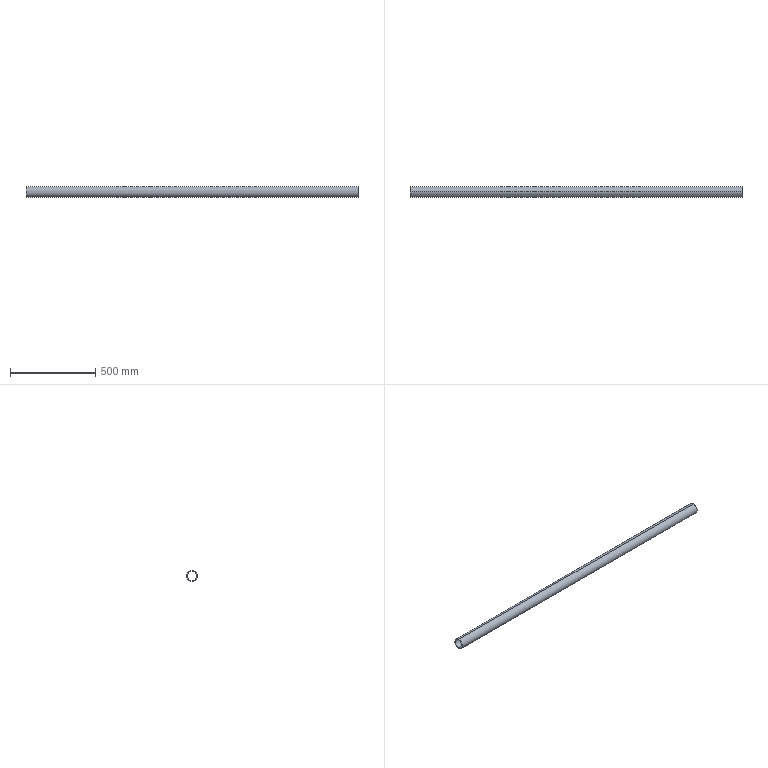Part | SolidWorks | features MoveFace 2, BaseBody 1 | 1 solid | 6 faces | box 1952 x 63 x 63 mm | volume 1103830 mm3 | cylinder 4 | plane 2 | commonest cylinder face diameters 57 x2 63 x2
STEP:
#1=CARTESIAN_POINT('',(976.,0.,28.5));
#2=VERTEX_POINT('',#1);
#3=CARTESIAN_POINT('',(976.,0.,-28.5));
#4=VERTEX_POINT('',#3);
#5=CARTESIAN_POINT('',(976.,0.,0.));
#6=DIRECTION('',(1.,0.,0.));
#7=DIRECTION('',(0.,0.,-1.));
#8=AXIS2_PLACEMENT_3D('',#5,#6,#7);
#9=CIRCLE('',#8,28.5);
#10=EDGE_CURVE('',#2,#4,#9,.T.);
#11=ORIENTED_EDGE('',*,*,#10,.T.);
#12=CARTESIAN_POINT('',(-976.,0.,-28.5));
#13=VERTEX_POINT('',#12);
#14=CARTESIAN_POINT('',(920.,0.,-28.5));
#15=DIRECTION('',(-1.,0.,0.));
#16=VECTOR('',#15,1000.);
#17=LINE('',#14,#16);
#18=EDGE_CURVE('',#4,#13,#17,.T.);
#19=ORIENTED_EDGE('',*,*,#18,.T.);
#20=CARTESIAN_POINT('',(-976.,0.,28.5));
#21=VERTEX_POINT('',#20);
#22=CARTESIAN_POINT('',(-976.,0.,0.));
#23=DIRECTION('',(1.,0.,0.));
#24=DIRECTION('',(0.,0.,-1.));
#25=AXIS2_PLACEMENT_3D('',#22,#23,#24);
#26=CIRCLE('',#25,28.5);
#27=EDGE_CURVE('',#21,#13,#26,.T.);
#28=ORIENTED_EDGE('',*,*,#27,.F.);
#29=CARTESIAN_POINT('',(920.,0.,28.5));
#30=DIRECTION('',(-1.,0.,0.));
#31=VECTOR('',#30,1000.);
#32=LINE('',#29,#31);
#33=EDGE_CURVE('',#2,#21,#32,.T.);
#34=ORIENTED_EDGE('',*,*,#33,.F.);
#35=EDGE_LOOP('',(#11,#19,#28,#34));
#36=FACE_OUTER_BOUND('',#35,.T.);
#37=CARTESIAN_POINT('',(920.,0.,0.));
#38=DIRECTION('',(-1.,0.,0.));
#39=DIRECTION('',(0.,0.,1.));
#40=AXIS2_PLACEMENT_3D('',#37,#38,#39);
#41=CYLINDRICAL_SURFACE('',#40,28.5);
#42=ADVANCED_FACE('',(#36),#41,.F.);
#43=CARTESIAN_POINT('',(976.,0.,-31.5));
#44=VERTEX_POINT('',#43);
#45=CARTESIAN_POINT('',(976.,0.,31.5));
#46=VERTEX_POINT('',#45);
#47=CARTESIAN_POINT('',(976.,0.,0.));
#48=DIRECTION('',(1.,0.,0.));
#49=DIRECTION('',(0.,0.,-1.));
#50=AXIS2_PLACEMENT_3D('',#47,#48,#49);
#51=CIRCLE('',#50,31.5);
#52=EDGE_CURVE('',#44,#46,#51,.T.);
#53=ORIENTED_EDGE('',*,*,#52,.F.);
#54=CARTESIAN_POINT('',(-976.,0.,-31.5));
#55=VERTEX_POINT('',#54);
#56=CARTESIAN_POINT('',(920.,0.,-31.5));
#57=DIRECTION('',(-1.,0.,0.));
#58=VECTOR('',#57,1000.);
#59=LINE('',#56,#58);
#60=EDGE_CURVE('',#44,#55,#59,.T.);
#61=ORIENTED_EDGE('',*,*,#60,.T.);
#62=CARTESIAN_POINT('',(-976.,0.,31.5));
#63=VERTEX_POINT('',#62);
#64=CARTESIAN_POINT('',(-976.,0.,0.));
#65=DIRECTION('',(1.,0.,0.));
#66=DIRECTION('',(0.,0.,-1.));
#67=AXIS2_PLACEMENT_3D('',#64,#65,#66);
#68=CIRCLE('',#67,31.5);
#69=EDGE_CURVE('',#55,#63,#68,.T.);
#70=ORIENTED_EDGE('',*,*,#69,.T.);
#71=CARTESIAN_POINT('',(920.,0.,31.5));
#72=DIRECTION('',(-1.,0.,0.));
#73=VECTOR('',#72,1000.);
#74=LINE('',#71,#73);
#75=EDGE_CURVE('',#46,#63,#74,.T.);
#76=ORIENTED_EDGE('',*,*,#75,.F.);
#77=EDGE_LOOP('',(#53,#61,#70,#76));
#78=FACE_OUTER_BOUND('',#77,.T.);
#79=CARTESIAN_POINT('',(920.,0.,0.));
#80=DIRECTION('',(-1.,0.,0.));
#81=DIRECTION('',(0.,0.,1.));
#82=AXIS2_PLACEMENT_3D('',#79,#80,#81);
#83=CYLINDRICAL_SURFACE('',#82,31.5);
#84=ADVANCED_FACE('',(#78),#83,.T.);
#85=CARTESIAN_POINT('',(976.,0.,0.));
#86=DIRECTION('',(1.,0.,0.));
#87=DIRECTION('',(0.,0.,-1.));
#88=AXIS2_PLACEMENT_3D('',#85,#86,#87);
#89=CIRCLE('',#88,31.5);
#90=EDGE_CURVE('',#46,#44,#89,.T.);
#91=ORIENTED_EDGE('',*,*,#90,.T.);
#92=ORIENTED_EDGE('',*,*,#52,.T.);
#93=EDGE_LOOP('',(#91,#92));
#94=FACE_OUTER_BOUND('',#93,.T.);
#95=ORIENTED_EDGE('',*,*,#10,.F.);
#96=CARTESIAN_POINT('',(976.,0.,0.));
#97=DIRECTION('',(1.,0.,0.));
#98=DIRECTION('',(0.,0.,-1.));
#99=AXIS2_PLACEMENT_3D('',#96,#97,#98);
#100=CIRCLE('',#99,28.5);
#101=EDGE_CURVE('',#4,#2,#100,.T.);
#102=ORIENTED_EDGE('',*,*,#101,.F.);
#103=EDGE_LOOP('',(#95,#102));
#104=FACE_BOUND('',#103,.T.);
#105=CARTESIAN_POINT('',(976.,0.,0.));
#106=DIRECTION('',(1.,0.,0.));
#107=DIRECTION('',(0.,0.,-1.));
#108=AXIS2_PLACEMENT_3D('',#105,#106,#107);
#109=PLANE('',#108);
#110=ADVANCED_FACE('',(#94,#104),#109,.T.);
#111=CARTESIAN_POINT('',(-976.,0.,0.));
#112=DIRECTION('',(1.,0.,0.));
#113=DIRECTION('',(0.,0.,-1.));
#114=AXIS2_PLACEMENT_3D('',#111,#112,#113);
#115=CIRCLE('',#114,31.5);
#116=EDGE_CURVE('',#63,#55,#115,.T.);
#117=ORIENTED_EDGE('',*,*,#116,.F.);
#118=ORIENTED_EDGE('',*,*,#69,.F.);
#119=EDGE_LOOP('',(#117,#118));
#120=FACE_OUTER_BOUND('',#119,.T.);
#121=ORIENTED_EDGE('',*,*,#27,.T.);
#122=CARTESIAN_POINT('',(-976.,0.,0.));
#123=DIRECTION('',(1.,0.,0.));
#124=DIRECTION('',(0.,0.,-1.));
#125=AXIS2_PLACEMENT_3D('',#122,#123,#124);
#126=CIRCLE('',#125,28.5);
#127=EDGE_CURVE('',#13,#21,#126,.T.);
#128=ORIENTED_EDGE('',*,*,#127,.T.);
#129=EDGE_LOOP('',(#121,#128));
#130=FACE_BOUND('',#129,.T.);
#131=CARTESIAN_POINT('',(-976.,0.,0.));
#132=DIRECTION('',(1.,0.,0.));
#133=DIRECTION('',(0.,0.,-1.));
#134=AXIS2_PLACEMENT_3D('',#131,#132,#133);
#135=PLANE('',#134);
#136=ADVANCED_FACE('',(#120,#130),#135,.F.);
#137=ORIENTED_EDGE('',*,*,#60,.F.);
#138=ORIENTED_EDGE('',*,*,#90,.F.);
#139=ORIENTED_EDGE('',*,*,#75,.T.);
#140=ORIENTED_EDGE('',*,*,#116,.T.);
#141=EDGE_LOOP('',(#137,#138,#139,#140));
#142=FACE_OUTER_BOUND('',#141,.T.);
#143=CARTESIAN_POINT('',(920.,0.,0.));
#144=DIRECTION('',(-1.,0.,0.));
#145=DIRECTION('',(0.,0.,1.));
#146=AXIS2_PLACEMENT_3D('',#143,#144,#145);
#147=CYLINDRICAL_SURFACE('',#146,31.5);
#148=ADVANCED_FACE('',(#142),#147,.T.);
#149=ORIENTED_EDGE('',*,*,#18,.F.);
#150=ORIENTED_EDGE('',*,*,#101,.T.);
#151=ORIENTED_EDGE('',*,*,#33,.T.);
#152=ORIENTED_EDGE('',*,*,#127,.F.);
#153=EDGE_LOOP('',(#149,#150,#151,#152));
#154=FACE_OUTER_BOUND('',#153,.T.);
#155=CARTESIAN_POINT('',(920.,0.,0.));
#156=DIRECTION('',(-1.,0.,0.));
#157=DIRECTION('',(0.,0.,1.));
#158=AXIS2_PLACEMENT_3D('',#155,#156,#157);
#159=CYLINDRICAL_SURFACE('',#158,28.5);
#160=ADVANCED_FACE('',(#154),#159,.F.);
#161=CLOSED_SHELL('',(#42,#84,#110,#136,#148,#160));
#162=MANIFOLD_SOLID_BREP('',#161);
#163=CARTESIAN_POINT('',(0.,0.,0.));
#164=DIRECTION('',(0.,0.,1.));
#165=DIRECTION('',(1.,0.,0.));
#166=AXIS2_PLACEMENT_3D('',#163,#164,#165);
#167=(LENGTH_UNIT()NAMED_UNIT(*)SI_UNIT(.MILLI.,.METRE.));
#168=UNCERTAINTY_MEASURE_WITH_UNIT(LENGTH_MEASURE(0.00001),#167,'','');
#169=(NAMED_UNIT(*)PLANE_ANGLE_UNIT()SI_UNIT($,.RADIAN.));
#170=(NAMED_UNIT(*)SI_UNIT($,.STERADIAN.)SOLID_ANGLE_UNIT());
#171=(GEOMETRIC_REPRESENTATION_CONTEXT(3)GLOBAL_UNCERTAINTY_ASSIGNED_CONTEXT((#168))GLOBAL_UNIT_ASSIGNED_CONTEXT((#167,#169,#170))REPRESENTATION_CONTEXT('',''));
#172=ADVANCED_BREP_SHAPE_REPRESENTATION('',(#162,#166),#171);